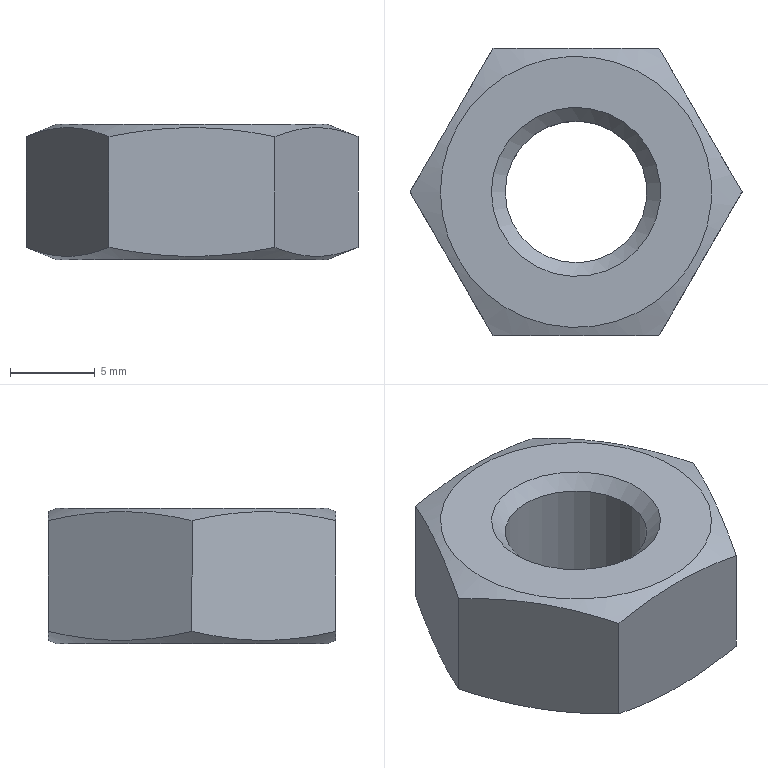Part | STEP file | 1_32 | 1 solid | 13 faces | box 19.63 x 17 x 8 mm | volume 1521 mm3 | plane 8 | cone 4 | cylinder 1 | commonest cylinder face diameters 8.376 x1
STEP:
#1=CARTESIAN_POINT('',(0.,0.,0.));
#2=DIRECTION('',(0.,0.,1.));
#3=DIRECTION('',(1.,0.,0.));
#4=AXIS2_PLACEMENT_3D('',#1,#2,#3);
#5=CARTESIAN_POINT('',(-4.188,0.,0.8119));
#6=VERTEX_POINT('',#5);
#7=CARTESIAN_POINT('',(0.,0.,0.8119));
#8=DIRECTION('',(0.,0.,-1.));
#9=DIRECTION('',(1.,0.,0.));
#10=AXIS2_PLACEMENT_3D('',#7,#8,#9);
#11=CIRCLE('',#10,4.188);
#12=CARTESIAN_POINT('',(0.,0.,0.4059));
#13=DIRECTION('',(0.,0.,-1.));
#14=DIRECTION('',(1.,0.,0.));
#15=AXIS2_PLACEMENT_3D('',#12,#13,#14);
#16=CONICAL_SURFACE('',#15,4.594,0.7854);
#17=CARTESIAN_POINT('',(0.,-0.4059));
#18=DIRECTION('',(1.,0.));
#19=VECTOR('',#18,1.);
#20=LINE('',#17,#19);
#21=(GEOMETRIC_REPRESENTATION_CONTEXT(2)PARAMETRIC_REPRESENTATION_CONTEXT()REPRESENTATION_CONTEXT('',''));
#22=DEFINITIONAL_REPRESENTATION('',(#20),#21);
#23=PCURVE('',#16,#22);
#24=CARTESIAN_POINT('',(0.,0.,4.));
#25=DIRECTION('',(0.,0.,-1.));
#26=DIRECTION('',(1.,0.,0.));
#27=AXIS2_PLACEMENT_3D('',#24,#25,#26);
#28=CYLINDRICAL_SURFACE('',#27,4.188);
#29=CARTESIAN_POINT('',(0.,3.188));
#30=DIRECTION('',(1.,0.));
#31=VECTOR('',#30,1.);
#32=LINE('',#29,#31);
#33=(GEOMETRIC_REPRESENTATION_CONTEXT(2)PARAMETRIC_REPRESENTATION_CONTEXT()REPRESENTATION_CONTEXT('',''));
#34=DEFINITIONAL_REPRESENTATION('',(#32),#33);
#35=PCURVE('',#28,#34);
#36=SURFACE_CURVE('',#11,(#23,#35),.PCURVE_S1.);
#37=EDGE_CURVE('',#6,#6,#36,.T.);
#38=ORIENTED_EDGE('',*,*,#37,.T.);
#39=CARTESIAN_POINT('',(-5.,0.,0.));
#40=VERTEX_POINT('',#39);
#41=CARTESIAN_POINT('',(-4.188,0.,0.8119));
#42=CARTESIAN_POINT('',(-5.,0.,0.));
#43=B_SPLINE_CURVE_WITH_KNOTS('',1,(#41,#42),.UNSPECIFIED.,.F.,.F.,(2,2),(-0.5741,0.5741),.PIECEWISE_BEZIER_KNOTS.);
#44=CARTESIAN_POINT('',(9.425,0.));
#45=DIRECTION('',(0.,1.));
#46=VECTOR('',#45,1.);
#47=LINE('',#44,#46);
#48=(GEOMETRIC_REPRESENTATION_CONTEXT(2)PARAMETRIC_REPRESENTATION_CONTEXT()REPRESENTATION_CONTEXT('',''));
#49=DEFINITIONAL_REPRESENTATION('',(#47),#48);
#50=PCURVE('',#16,#49);
#51=CARTESIAN_POINT('',(3.142,0.));
#52=DIRECTION('',(0.,1.));
#53=VECTOR('',#52,1.);
#54=LINE('',#51,#53);
#55=(GEOMETRIC_REPRESENTATION_CONTEXT(2)PARAMETRIC_REPRESENTATION_CONTEXT()REPRESENTATION_CONTEXT('',''));
#56=DEFINITIONAL_REPRESENTATION('',(#54),#55);
#57=PCURVE('',#16,#56);
#58=SEAM_CURVE('',#43,(#50,#57),.PCURVE_S1.);
#59=EDGE_CURVE('',#6,#40,#58,.T.);
#60=ORIENTED_EDGE('',*,*,#59,.T.);
#61=CARTESIAN_POINT('',(0.,0.,0.));
#62=DIRECTION('',(0.,0.,-1.));
#63=DIRECTION('',(1.,0.,0.));
#64=AXIS2_PLACEMENT_3D('',#61,#62,#63);
#65=CIRCLE('',#64,5.);
#66=CARTESIAN_POINT('',(0.,0.4059));
#67=DIRECTION('',(1.,0.));
#68=VECTOR('',#67,1.);
#69=LINE('',#66,#68);
#70=(GEOMETRIC_REPRESENTATION_CONTEXT(2)PARAMETRIC_REPRESENTATION_CONTEXT()REPRESENTATION_CONTEXT('',''));
#71=DEFINITIONAL_REPRESENTATION('',(#69),#70);
#72=PCURVE('',#16,#71);
#73=CARTESIAN_POINT('',(0.,0.,0.));
#74=DIRECTION('',(0.,0.,1.));
#75=DIRECTION('',(1.,0.,0.));
#76=AXIS2_PLACEMENT_3D('',#73,#74,#75);
#77=PLANE('',#76);
#78=CARTESIAN_POINT('',(5.,0.));
#79=CARTESIAN_POINT('',(5.,-8.66));
#80=CARTESIAN_POINT('',(-2.5,-4.33));
#81=CARTESIAN_POINT('',(-10.,0.));
#82=CARTESIAN_POINT('',(-2.5,4.33));
#83=CARTESIAN_POINT('',(5.,8.66));
#84=CARTESIAN_POINT('',(5.,0.));
#85=(BOUNDED_CURVE()B_SPLINE_CURVE(2,(#78,#79,#80,#81,#82,#83,#84),.UNSPECIFIED.,.T.,.F.)B_SPLINE_CURVE_WITH_KNOTS((1,2,2,2,2,1),(-2.094,0.,2.094,4.189,6.283,8.378),.UNSPECIFIED.)CURVE()GEOMETRIC_REPRESENTATION_ITEM()RATIONAL_B_SPLINE_CURVE((1.,0.5,1.,0.5,1.,0.5,1.))REPRESENTATION_ITEM(''));
#86=(GEOMETRIC_REPRESENTATION_CONTEXT(2)PARAMETRIC_REPRESENTATION_CONTEXT()REPRESENTATION_CONTEXT('',''));
#87=DEFINITIONAL_REPRESENTATION('',(#85),#86);
#88=PCURVE('',#77,#87);
#89=SURFACE_CURVE('',#65,(#72,#88),.PCURVE_S1.);
#90=EDGE_CURVE('',#40,#40,#89,.T.);
#91=ORIENTED_EDGE('',*,*,#90,.F.);
#92=ORIENTED_EDGE('',*,*,#59,.F.);
#93=EDGE_LOOP('',(#38,#60,#91,#92));
#94=FACE_BOUND('',#93,.F.);
#95=ADVANCED_FACE('',(#94),#16,.F.);
#96=CARTESIAN_POINT('',(-8.015,0.,0.));
#97=VERTEX_POINT('',#96);
#98=CARTESIAN_POINT('',(0.,0.,0.));
#99=DIRECTION('',(0.,0.,1.));
#100=DIRECTION('',(1.,0.,0.));
#101=AXIS2_PLACEMENT_3D('',#98,#99,#100);
#102=CIRCLE('',#101,8.015);
#103=CARTESIAN_POINT('',(0.,0.));
#104=DIRECTION('',(1.,0.));
#105=AXIS2_PLACEMENT_2D('',#103,#104);
#106=CIRCLE('',#105,8.015);
#107=(GEOMETRIC_REPRESENTATION_CONTEXT(2)PARAMETRIC_REPRESENTATION_CONTEXT()REPRESENTATION_CONTEXT('',''));
#108=DEFINITIONAL_REPRESENTATION('',(#106),#107);
#109=PCURVE('',#77,#108);
#110=CARTESIAN_POINT('',(0.,0.,0.3636));
#111=DIRECTION('',(0.,0.,1.));
#112=DIRECTION('',(1.,0.,0.));
#113=AXIS2_PLACEMENT_3D('',#110,#111,#112);
#114=CONICAL_SURFACE('',#113,8.915,1.187);
#115=CARTESIAN_POINT('',(0.,-0.3636));
#116=DIRECTION('',(1.,0.));
#117=VECTOR('',#116,1.);
#118=LINE('',#115,#117);
#119=(GEOMETRIC_REPRESENTATION_CONTEXT(2)PARAMETRIC_REPRESENTATION_CONTEXT()REPRESENTATION_CONTEXT('',''));
#120=DEFINITIONAL_REPRESENTATION('',(#118),#119);
#121=PCURVE('',#114,#120);
#122=SURFACE_CURVE('',#102,(#109,#121),.PCURVE_S1.);
#123=EDGE_CURVE('',#97,#97,#122,.T.);
#124=ORIENTED_EDGE('',*,*,#123,.F.);
#125=EDGE_LOOP('',(#124));
#126=FACE_BOUND('',#125,.T.);
#127=ORIENTED_EDGE('',*,*,#90,.F.);
#128=EDGE_LOOP('',(#127));
#129=FACE_BOUND('',#128,.T.);
#130=ADVANCED_FACE('',(#126,#129),#77,.F.);
#131=CARTESIAN_POINT('',(-4.188,0.,7.188));
#132=VERTEX_POINT('',#131);
#133=CARTESIAN_POINT('',(0.,0.,7.188));
#134=DIRECTION('',(0.,0.,1.));
#135=DIRECTION('',(-1.,0.,0.));
#136=AXIS2_PLACEMENT_3D('',#133,#134,#135);
#137=CIRCLE('',#136,4.188);
#138=CARTESIAN_POINT('',(9.425,-3.188));
#139=DIRECTION('',(-1.,0.));
#140=VECTOR('',#139,1.);
#141=LINE('',#138,#140);
#142=(GEOMETRIC_REPRESENTATION_CONTEXT(2)PARAMETRIC_REPRESENTATION_CONTEXT()REPRESENTATION_CONTEXT('',''));
#143=DEFINITIONAL_REPRESENTATION('',(#141),#142);
#144=PCURVE('',#28,#143);
#145=CARTESIAN_POINT('',(0.,0.,7.594));
#146=DIRECTION('',(0.,0.,1.));
#147=DIRECTION('',(-1.,0.,0.));
#148=AXIS2_PLACEMENT_3D('',#145,#146,#147);
#149=CONICAL_SURFACE('',#148,4.594,0.7854);
#150=CARTESIAN_POINT('',(0.,-0.4059));
#151=DIRECTION('',(1.,0.));
#152=VECTOR('',#151,1.);
#153=LINE('',#150,#152);
#154=(GEOMETRIC_REPRESENTATION_CONTEXT(2)PARAMETRIC_REPRESENTATION_CONTEXT()REPRESENTATION_CONTEXT('',''));
#155=DEFINITIONAL_REPRESENTATION('',(#153),#154);
#156=PCURVE('',#149,#155);
#157=SURFACE_CURVE('',#137,(#144,#156),.PCURVE_S1.);
#158=EDGE_CURVE('',#132,#132,#157,.T.);
#159=ORIENTED_EDGE('',*,*,#158,.F.);
#160=CARTESIAN_POINT('',(-4.188,0.,7.188));
#161=CARTESIAN_POINT('',(-4.188,0.,0.8119));
#162=B_SPLINE_CURVE_WITH_KNOTS('',1,(#160,#161),.UNSPECIFIED.,.F.,.F.,(2,2),(-3.188,3.188),.PIECEWISE_BEZIER_KNOTS.);
#163=CARTESIAN_POINT('',(9.425,0.));
#164=DIRECTION('',(0.,1.));
#165=VECTOR('',#164,1.);
#166=LINE('',#163,#165);
#167=(GEOMETRIC_REPRESENTATION_CONTEXT(2)PARAMETRIC_REPRESENTATION_CONTEXT()REPRESENTATION_CONTEXT('',''));
#168=DEFINITIONAL_REPRESENTATION('',(#166),#167);
#169=PCURVE('',#28,#168);
#170=CARTESIAN_POINT('',(3.142,0.));
#171=DIRECTION('',(0.,1.));
#172=VECTOR('',#171,1.);
#173=LINE('',#170,#172);
#174=(GEOMETRIC_REPRESENTATION_CONTEXT(2)PARAMETRIC_REPRESENTATION_CONTEXT()REPRESENTATION_CONTEXT('',''));
#175=DEFINITIONAL_REPRESENTATION('',(#173),#174);
#176=PCURVE('',#28,#175);
#177=SEAM_CURVE('',#162,(#169,#176),.PCURVE_S1.);
#178=EDGE_CURVE('',#132,#6,#177,.T.);
#179=ORIENTED_EDGE('',*,*,#178,.T.);
#180=ORIENTED_EDGE('',*,*,#37,.F.);
#181=ORIENTED_EDGE('',*,*,#178,.F.);
#182=EDGE_LOOP('',(#159,#179,#180,#181));
#183=FACE_BOUND('',#182,.F.);
#184=ADVANCED_FACE('',(#183),#28,.F.);
#185=CARTESIAN_POINT('',(-9.815,0.,0.7273));
#186=VERTEX_POINT('',#185);
#187=CARTESIAN_POINT('',(-4.907,8.5,0.7273));
#188=VERTEX_POINT('',#187);
#189=CARTESIAN_POINT('',(-21.724,-20.628,8.865));
#190=CARTESIAN_POINT('',(-7.361,4.25,-2.264));
#191=CARTESIAN_POINT('',(7.002,29.128,8.865));
#192=(BOUNDED_CURVE()B_SPLINE_CURVE(2,(#189,#190,#191),.UNSPECIFIED.,.F.,.F.)B_SPLINE_CURVE_WITH_KNOTS((3,3),(0.,6.001),.PIECEWISE_BEZIER_KNOTS.)CURVE()GEOMETRIC_REPRESENTATION_ITEM()RATIONAL_B_SPLINE_CURVE((1.,3.524,1.))REPRESENTATION_ITEM(''));
#193=CARTESIAN_POINT('',(9.425,0.3636));
#194=CARTESIAN_POINT('',(9.41,0.329));
#195=CARTESIAN_POINT('',(9.379,0.2637));
#196=CARTESIAN_POINT('',(9.333,0.1773));
#197=CARTESIAN_POINT('',(9.286,0.1018));
#198=CARTESIAN_POINT('',(9.239,0.03643));
#199=CARTESIAN_POINT('',(9.191,-0.01926));
#200=CARTESIAN_POINT('',(9.144,-0.0657));
#201=CARTESIAN_POINT('',(9.095,-0.1032));
#202=CARTESIAN_POINT('',(9.047,-0.1322));
#203=CARTESIAN_POINT('',(8.999,-0.1527));
#204=CARTESIAN_POINT('',(8.95,-0.1649));
#205=CARTESIAN_POINT('',(8.901,-0.169));
#206=CARTESIAN_POINT('',(8.852,-0.1649));
#207=CARTESIAN_POINT('',(8.804,-0.1527));
#208=CARTESIAN_POINT('',(8.755,-0.1322));
#209=CARTESIAN_POINT('',(8.707,-0.1032));
#210=CARTESIAN_POINT('',(8.659,-0.0657));
#211=CARTESIAN_POINT('',(8.611,-0.01926));
#212=CARTESIAN_POINT('',(8.563,0.03643));
#213=CARTESIAN_POINT('',(8.516,0.1018));
#214=CARTESIAN_POINT('',(8.469,0.1773));
#215=CARTESIAN_POINT('',(8.423,0.2637));
#216=CARTESIAN_POINT('',(8.393,0.329));
#217=CARTESIAN_POINT('',(8.378,0.3636));
#218=B_SPLINE_CURVE_WITH_KNOTS('',3,(#193,#194,#195,#196,#197,#198,#199,#200,#201,#202,#203,#204,#205,#206,#207,#208,#209,#210,#211,#212,#213,#214,#215,#216,#217),.UNSPECIFIED.,.F.,.F.,(4,1,1,1,1,1,1,1,1,1,1,1,1,1,1,1,1,1,1,1,1,1,4),(1.924,2.022,2.12,2.218,2.316,2.414,2.511,2.609,2.707,2.805,2.903,3.001,3.098,3.196,3.294,3.392,3.49,3.588,3.686,3.783,3.881,3.979,4.077),.QUASI_UNIFORM_KNOTS.);
#219=(GEOMETRIC_REPRESENTATION_CONTEXT(2)PARAMETRIC_REPRESENTATION_CONTEXT()REPRESENTATION_CONTEXT('',''));
#220=DEFINITIONAL_REPRESENTATION('',(#218),#219);
#221=PCURVE('',#114,#220);
#222=CARTESIAN_POINT('',(-9.815,0.,0.));
#223=DIRECTION('',(-0.866,0.5,0.));
#224=DIRECTION('',(0.,0.,1.));
#225=AXIS2_PLACEMENT_3D('',#222,#223,#224);
#226=PLANE('',#225);
#227=CARTESIAN_POINT('',(8.865,-23.819));
#228=CARTESIAN_POINT('',(-2.264,4.907));
#229=CARTESIAN_POINT('',(8.865,33.634));
#230=(BOUNDED_CURVE()B_SPLINE_CURVE(2,(#227,#228,#229),.UNSPECIFIED.,.F.,.F.)B_SPLINE_CURVE_WITH_KNOTS((3,3),(0.,6.001),.PIECEWISE_BEZIER_KNOTS.)CURVE()GEOMETRIC_REPRESENTATION_ITEM()RATIONAL_B_SPLINE_CURVE((1.,3.524,1.))REPRESENTATION_ITEM(''));
#231=(GEOMETRIC_REPRESENTATION_CONTEXT(2)PARAMETRIC_REPRESENTATION_CONTEXT()REPRESENTATION_CONTEXT('',''));
#232=DEFINITIONAL_REPRESENTATION('',(#230),#231);
#233=PCURVE('',#226,#232);
#234=SURFACE_CURVE('',#192,(#221,#233),.PCURVE_S1.);
#235=EDGE_CURVE('',#186,#188,#234,.T.);
#236=ORIENTED_EDGE('',*,*,#235,.T.);
#237=CARTESIAN_POINT('',(4.907,8.5,0.7273));
#238=VERTEX_POINT('',#237);
#239=CARTESIAN_POINT('',(-28.727,8.5,8.865));
#240=CARTESIAN_POINT('',(0.,8.5,-2.264));
#241=CARTESIAN_POINT('',(28.727,8.5,8.865));
#242=(BOUNDED_CURVE()B_SPLINE_CURVE(2,(#239,#240,#241),.UNSPECIFIED.,.F.,.F.)B_SPLINE_CURVE_WITH_KNOTS((3,3),(0.,6.001),.PIECEWISE_BEZIER_KNOTS.)CURVE()GEOMETRIC_REPRESENTATION_ITEM()RATIONAL_B_SPLINE_CURVE((1.,3.524,1.))REPRESENTATION_ITEM(''));
#243=CARTESIAN_POINT('',(8.378,0.3636));
#244=CARTESIAN_POINT('',(8.362,0.329));
#245=CARTESIAN_POINT('',(8.332,0.2637));
#246=CARTESIAN_POINT('',(8.286,0.1773));
#247=CARTESIAN_POINT('',(8.239,0.1018));
#248=CARTESIAN_POINT('',(8.192,0.03643));
#249=CARTESIAN_POINT('',(8.144,-0.01926));
#250=CARTESIAN_POINT('',(8.096,-0.0657));
#251=CARTESIAN_POINT('',(8.048,-0.1032));
#252=CARTESIAN_POINT('',(8.,-0.1322));
#253=CARTESIAN_POINT('',(7.951,-0.1527));
#254=CARTESIAN_POINT('',(7.903,-0.1649));
#255=CARTESIAN_POINT('',(7.854,-0.169));
#256=CARTESIAN_POINT('',(7.805,-0.1649));
#257=CARTESIAN_POINT('',(7.757,-0.1527));
#258=CARTESIAN_POINT('',(7.708,-0.1322));
#259=CARTESIAN_POINT('',(7.66,-0.1032));
#260=CARTESIAN_POINT('',(7.612,-0.0657));
#261=CARTESIAN_POINT('',(7.564,-0.01926));
#262=CARTESIAN_POINT('',(7.516,0.03643));
#263=CARTESIAN_POINT('',(7.469,0.1018));
#264=CARTESIAN_POINT('',(7.422,0.1773));
#265=CARTESIAN_POINT('',(7.376,0.2637));
#266=CARTESIAN_POINT('',(7.346,0.329));
#267=CARTESIAN_POINT('',(7.33,0.3636));
#268=B_SPLINE_CURVE_WITH_KNOTS('',3,(#243,#244,#245,#246,#247,#248,#249,#250,#251,#252,#253,#254,#255,#256,#257,#258,#259,#260,#261,#262,#263,#264,#265,#266,#267),.UNSPECIFIED.,.F.,.F.,(4,1,1,1,1,1,1,1,1,1,1,1,1,1,1,1,1,1,1,1,1,1,4),(1.924,2.022,2.12,2.218,2.316,2.414,2.511,2.609,2.707,2.805,2.903,3.001,3.098,3.196,3.294,3.392,3.49,3.588,3.686,3.783,3.881,3.979,4.077),.QUASI_UNIFORM_KNOTS.);
#269=(GEOMETRIC_REPRESENTATION_CONTEXT(2)PARAMETRIC_REPRESENTATION_CONTEXT()REPRESENTATION_CONTEXT('',''));
#270=DEFINITIONAL_REPRESENTATION('',(#268),#269);
#271=PCURVE('',#114,#270);
#272=CARTESIAN_POINT('',(-4.907,8.5,0.));
#273=DIRECTION('',(0.,1.,0.));
#274=DIRECTION('',(0.,0.,1.));
#275=AXIS2_PLACEMENT_3D('',#272,#273,#274);
#276=PLANE('',#275);
#277=CARTESIAN_POINT('',(8.865,-23.819));
#278=CARTESIAN_POINT('',(-2.264,4.907));
#279=CARTESIAN_POINT('',(8.865,33.634));
#280=(BOUNDED_CURVE()B_SPLINE_CURVE(2,(#277,#278,#279),.UNSPECIFIED.,.F.,.F.)B_SPLINE_CURVE_WITH_KNOTS((3,3),(0.,6.001),.PIECEWISE_BEZIER_KNOTS.)CURVE()GEOMETRIC_REPRESENTATION_ITEM()RATIONAL_B_SPLINE_CURVE((1.,3.524,1.))REPRESENTATION_ITEM(''));
#281=(GEOMETRIC_REPRESENTATION_CONTEXT(2)PARAMETRIC_REPRESENTATION_CONTEXT()REPRESENTATION_CONTEXT('',''));
#282=DEFINITIONAL_REPRESENTATION('',(#280),#281);
#283=PCURVE('',#276,#282);
#284=SURFACE_CURVE('',#242,(#271,#283),.PCURVE_S1.);
#285=EDGE_CURVE('',#188,#238,#284,.T.);
#286=ORIENTED_EDGE('',*,*,#285,.T.);
#287=CARTESIAN_POINT('',(9.815,0.,0.7273));
#288=VERTEX_POINT('',#287);
#289=CARTESIAN_POINT('',(-7.002,29.128,8.865));
#290=CARTESIAN_POINT('',(7.361,4.25,-2.264));
#291=CARTESIAN_POINT('',(21.724,-20.628,8.865));
#292=(BOUNDED_CURVE()B_SPLINE_CURVE(2,(#289,#290,#291),.UNSPECIFIED.,.F.,.F.)B_SPLINE_CURVE_WITH_KNOTS((3,3),(0.,6.001),.PIECEWISE_BEZIER_KNOTS.)CURVE()GEOMETRIC_REPRESENTATION_ITEM()RATIONAL_B_SPLINE_CURVE((1.,3.524,1.))REPRESENTATION_ITEM(''));
#293=CARTESIAN_POINT('',(7.33,0.3636));
#294=CARTESIAN_POINT('',(7.315,0.329));
#295=CARTESIAN_POINT('',(7.285,0.2637));
#296=CARTESIAN_POINT('',(7.238,0.1773));
#297=CARTESIAN_POINT('',(7.192,0.1018));
#298=CARTESIAN_POINT('',(7.145,0.03643));
#299=CARTESIAN_POINT('',(7.097,-0.01926));
#300=CARTESIAN_POINT('',(7.049,-0.0657));
#301=CARTESIAN_POINT('',(7.001,-0.1032));
#302=CARTESIAN_POINT('',(6.953,-0.1322));
#303=CARTESIAN_POINT('',(6.904,-0.1527));
#304=CARTESIAN_POINT('',(6.856,-0.1649));
#305=CARTESIAN_POINT('',(6.807,-0.169));
#306=CARTESIAN_POINT('',(6.758,-0.1649));
#307=CARTESIAN_POINT('',(6.709,-0.1527));
#308=CARTESIAN_POINT('',(6.661,-0.1322));
#309=CARTESIAN_POINT('',(6.612,-0.1032));
#310=CARTESIAN_POINT('',(6.564,-0.0657));
#311=CARTESIAN_POINT('',(6.516,-0.01926));
#312=CARTESIAN_POINT('',(6.469,0.03643));
#313=CARTESIAN_POINT('',(6.422,0.1018));
#314=CARTESIAN_POINT('',(6.375,0.1773));
#315=CARTESIAN_POINT('',(6.329,0.2637));
#316=CARTESIAN_POINT('',(6.298,0.329));
#317=CARTESIAN_POINT('',(6.283,0.3636));
#318=B_SPLINE_CURVE_WITH_KNOTS('',3,(#293,#294,#295,#296,#297,#298,#299,#300,#301,#302,#303,#304,#305,#306,#307,#308,#309,#310,#311,#312,#313,#314,#315,#316,#317),.UNSPECIFIED.,.F.,.F.,(4,1,1,1,1,1,1,1,1,1,1,1,1,1,1,1,1,1,1,1,1,1,4),(1.924,2.022,2.12,2.218,2.316,2.414,2.511,2.609,2.707,2.805,2.903,3.001,3.098,3.196,3.294,3.392,3.49,3.588,3.686,3.783,3.881,3.979,4.077),.QUASI_UNIFORM_KNOTS.);
#319=(GEOMETRIC_REPRESENTATION_CONTEXT(2)PARAMETRIC_REPRESENTATION_CONTEXT()REPRESENTATION_CONTEXT('',''));
#320=DEFINITIONAL_REPRESENTATION('',(#318),#319);
#321=PCURVE('',#114,#320);
#322=CARTESIAN_POINT('',(4.907,8.5,0.));
#323=DIRECTION('',(0.866,0.5,0.));
#324=DIRECTION('',(0.,0.,-1.));
#325=AXIS2_PLACEMENT_3D('',#322,#323,#324);
#326=PLANE('',#325);
#327=CARTESIAN_POINT('',(-8.865,23.819));
#328=CARTESIAN_POINT('',(2.264,-4.907));
#329=CARTESIAN_POINT('',(-8.865,-33.634));
#330=(BOUNDED_CURVE()B_SPLINE_CURVE(2,(#327,#328,#329),.UNSPECIFIED.,.F.,.F.)B_SPLINE_CURVE_WITH_KNOTS((3,3),(0.,6.001),.PIECEWISE_BEZIER_KNOTS.)CURVE()GEOMETRIC_REPRESENTATION_ITEM()RATIONAL_B_SPLINE_CURVE((1.,3.524,1.))REPRESENTATION_ITEM(''));
#331=(GEOMETRIC_REPRESENTATION_CONTEXT(2)PARAMETRIC_REPRESENTATION_CONTEXT()REPRESENTATION_CONTEXT('',''));
#332=DEFINITIONAL_REPRESENTATION('',(#330),#331);
#333=PCURVE('',#326,#332);
#334=SURFACE_CURVE('',#292,(#321,#333),.PCURVE_S1.);
#335=EDGE_CURVE('',#238,#288,#334,.T.);
#336=ORIENTED_EDGE('',*,*,#335,.T.);
#337=CARTESIAN_POINT('',(4.907,-8.5,0.7273));
#338=VERTEX_POINT('',#337);
#339=CARTESIAN_POINT('',(21.724,20.628,8.865));
#340=CARTESIAN_POINT('',(7.361,-4.25,-2.264));
#341=CARTESIAN_POINT('',(-7.002,-29.128,8.865));
#342=(BOUNDED_CURVE()B_SPLINE_CURVE(2,(#339,#340,#341),.UNSPECIFIED.,.F.,.F.)B_SPLINE_CURVE_WITH_KNOTS((3,3),(0.,6.001),.PIECEWISE_BEZIER_KNOTS.)CURVE()GEOMETRIC_REPRESENTATION_ITEM()RATIONAL_B_SPLINE_CURVE((1.,3.524,1.))REPRESENTATION_ITEM(''));
#343=CARTESIAN_POINT('',(6.283,0.3636));
#344=CARTESIAN_POINT('',(6.268,0.329));
#345=CARTESIAN_POINT('',(6.238,0.2637));
#346=CARTESIAN_POINT('',(6.191,0.1773));
#347=CARTESIAN_POINT('',(6.145,0.1018));
#348=CARTESIAN_POINT('',(6.097,0.03643));
#349=CARTESIAN_POINT('',(6.05,-0.01926));
#350=CARTESIAN_POINT('',(6.002,-0.0657));
#351=CARTESIAN_POINT('',(5.954,-0.1032));
#352=CARTESIAN_POINT('',(5.906,-0.1322));
#353=CARTESIAN_POINT('',(5.857,-0.1527));
#354=CARTESIAN_POINT('',(5.808,-0.1649));
#355=CARTESIAN_POINT('',(5.76,-0.169));
#356=CARTESIAN_POINT('',(5.711,-0.1649));
#357=CARTESIAN_POINT('',(5.662,-0.1527));
#358=CARTESIAN_POINT('',(5.614,-0.1322));
#359=CARTESIAN_POINT('',(5.565,-0.1032));
#360=CARTESIAN_POINT('',(5.517,-0.0657));
#361=CARTESIAN_POINT('',(5.469,-0.01926));
#362=CARTESIAN_POINT('',(5.422,0.03643));
#363=CARTESIAN_POINT('',(5.375,0.1018));
#364=CARTESIAN_POINT('',(5.328,0.1773));
#365=CARTESIAN_POINT('',(5.282,0.2637));
#366=CARTESIAN_POINT('',(5.251,0.329));
#367=CARTESIAN_POINT('',(5.236,0.3636));
#368=B_SPLINE_CURVE_WITH_KNOTS('',3,(#343,#344,#345,#346,#347,#348,#349,#350,#351,#352,#353,#354,#355,#356,#357,#358,#359,#360,#361,#362,#363,#364,#365,#366,#367),.UNSPECIFIED.,.F.,.F.,(4,1,1,1,1,1,1,1,1,1,1,1,1,1,1,1,1,1,1,1,1,1,4),(1.924,2.022,2.12,2.218,2.316,2.414,2.511,2.609,2.707,2.805,2.903,3.001,3.098,3.196,3.294,3.392,3.49,3.588,3.686,3.783,3.881,3.979,4.077),.QUASI_UNIFORM_KNOTS.);
#369=(GEOMETRIC_REPRESENTATION_CONTEXT(2)PARAMETRIC_REPRESENTATION_CONTEXT()REPRESENTATION_CONTEXT('',''));
#370=DEFINITIONAL_REPRESENTATION('',(#368),#369);
#371=PCURVE('',#114,#370);
#372=CARTESIAN_POINT('',(9.815,0.,0.));
#373=DIRECTION('',(0.866,-0.5,0.));
#374=DIRECTION('',(0.,0.,-1.));
#375=AXIS2_PLACEMENT_3D('',#372,#373,#374);
#376=PLANE('',#375);
#377=CARTESIAN_POINT('',(-8.865,23.819));
#378=CARTESIAN_POINT('',(2.264,-4.907));
#379=CARTESIAN_POINT('',(-8.865,-33.634));
#380=(BOUNDED_CURVE()B_SPLINE_CURVE(2,(#377,#378,#379),.UNSPECIFIED.,.F.,.F.)B_SPLINE_CURVE_WITH_KNOTS((3,3),(0.,6.001),.PIECEWISE_BEZIER_KNOTS.)CURVE()GEOMETRIC_REPRESENTATION_ITEM()RATIONAL_B_SPLINE_CURVE((1.,3.524,1.))REPRESENTATION_ITEM(''));
#381=(GEOMETRIC_REPRESENTATION_CONTEXT(2)PARAMETRIC_REPRESENTATION_CONTEXT()REPRESENTATION_CONTEXT('',''));
#382=DEFINITIONAL_REPRESENTATION('',(#380),#381);
#383=PCURVE('',#376,#382);
#384=SURFACE_CURVE('',#342,(#371,#383),.PCURVE_S1.);
#385=EDGE_CURVE('',#288,#338,#384,.T.);
#386=ORIENTED_EDGE('',*,*,#385,.T.);
#387=CARTESIAN_POINT('',(-4.907,-8.5,0.7273));
#388=VERTEX_POINT('',#387);
#389=CARTESIAN_POINT('',(28.727,-8.5,8.865));
#390=CARTESIAN_POINT('',(0.,-8.5,-2.264));
#391=CARTESIAN_POINT('',(-28.727,-8.5,8.865));
#392=(BOUNDED_CURVE()B_SPLINE_CURVE(2,(#389,#390,#391),.UNSPECIFIED.,.F.,.F.)B_SPLINE_CURVE_WITH_KNOTS((3,3),(0.,6.001),.PIECEWISE_BEZIER_KNOTS.)CURVE()GEOMETRIC_REPRESENTATION_ITEM()RATIONAL_B_SPLINE_CURVE((1.,3.524,1.))REPRESENTATION_ITEM(''));
#393=CARTESIAN_POINT('',(5.236,0.3636));
#394=CARTESIAN_POINT('',(5.221,0.329));
#395=CARTESIAN_POINT('',(5.19,0.2637));
#396=CARTESIAN_POINT('',(5.144,0.1773));
#397=CARTESIAN_POINT('',(5.097,0.1018));
#398=CARTESIAN_POINT('',(5.05,0.03643));
#399=CARTESIAN_POINT('',(5.003,-0.01926));
#400=CARTESIAN_POINT('',(4.955,-0.0657));
#401=CARTESIAN_POINT('',(4.907,-0.1032));
#402=CARTESIAN_POINT('',(4.858,-0.1322));
#403=CARTESIAN_POINT('',(4.81,-0.1527));
#404=CARTESIAN_POINT('',(4.761,-0.1649));
#405=CARTESIAN_POINT('',(4.712,-0.169));
#406=CARTESIAN_POINT('',(4.664,-0.1649));
#407=CARTESIAN_POINT('',(4.615,-0.1527));
#408=CARTESIAN_POINT('',(4.566,-0.1322));
#409=CARTESIAN_POINT('',(4.518,-0.1032));
#410=CARTESIAN_POINT('',(4.47,-0.0657));
#411=CARTESIAN_POINT('',(4.422,-0.01926));
#412=CARTESIAN_POINT('',(4.375,0.03643));
#413=CARTESIAN_POINT('',(4.327,0.1018));
#414=CARTESIAN_POINT('',(4.281,0.1773));
#415=CARTESIAN_POINT('',(4.234,0.2637));
#416=CARTESIAN_POINT('',(4.204,0.329));
#417=CARTESIAN_POINT('',(4.189,0.3636));
#418=B_SPLINE_CURVE_WITH_KNOTS('',3,(#393,#394,#395,#396,#397,#398,#399,#400,#401,#402,#403,#404,#405,#406,#407,#408,#409,#410,#411,#412,#413,#414,#415,#416,#417),.UNSPECIFIED.,.F.,.F.,(4,1,1,1,1,1,1,1,1,1,1,1,1,1,1,1,1,1,1,1,1,1,4),(1.924,2.022,2.12,2.218,2.316,2.414,2.511,2.609,2.707,2.805,2.903,3.001,3.098,3.196,3.294,3.392,3.49,3.588,3.686,3.783,3.881,3.979,4.077),.QUASI_UNIFORM_KNOTS.);
#419=(GEOMETRIC_REPRESENTATION_CONTEXT(2)PARAMETRIC_REPRESENTATION_CONTEXT()REPRESENTATION_CONTEXT('',''));
#420=DEFINITIONAL_REPRESENTATION('',(#418),#419);
#421=PCURVE('',#114,#420);
#422=CARTESIAN_POINT('',(4.907,-8.5,0.));
#423=DIRECTION('',(0.,-1.,0.));
#424=DIRECTION('',(0.,0.,-1.));
#425=AXIS2_PLACEMENT_3D('',#422,#423,#424);
#426=PLANE('',#425);
#427=CARTESIAN_POINT('',(-8.865,23.819));
#428=CARTESIAN_POINT('',(2.264,-4.907));
#429=CARTESIAN_POINT('',(-8.865,-33.634));
#430=(BOUNDED_CURVE()B_SPLINE_CURVE(2,(#427,#428,#429),.UNSPECIFIED.,.F.,.F.)B_SPLINE_CURVE_WITH_KNOTS((3,3),(0.,6.001),.PIECEWISE_BEZIER_KNOTS.)CURVE()GEOMETRIC_REPRESENTATION_ITEM()RATIONAL_B_SPLINE_CURVE((1.,3.524,1.))REPRESENTATION_ITEM(''));
#431=(GEOMETRIC_REPRESENTATION_CONTEXT(2)PARAMETRIC_REPRESENTATION_CONTEXT()REPRESENTATION_CONTEXT('',''));
#432=DEFINITIONAL_REPRESENTATION('',(#430),#431);
#433=PCURVE('',#426,#432);
#434=SURFACE_CURVE('',#392,(#421,#433),.PCURVE_S1.);
#435=EDGE_CURVE('',#338,#388,#434,.T.);
#436=ORIENTED_EDGE('',*,*,#435,.T.);
#437=CARTESIAN_POINT('',(7.002,-29.128,8.865));
#438=CARTESIAN_POINT('',(-7.361,-4.25,-2.264));
#439=CARTESIAN_POINT('',(-21.724,20.628,8.865));
#440=(BOUNDED_CURVE()B_SPLINE_CURVE(2,(#437,#438,#439),.UNSPECIFIED.,.F.,.F.)B_SPLINE_CURVE_WITH_KNOTS((3,3),(0.,6.001),.PIECEWISE_BEZIER_KNOTS.)CURVE()GEOMETRIC_REPRESENTATION_ITEM()RATIONAL_B_SPLINE_CURVE((1.,3.524,1.))REPRESENTATION_ITEM(''));
#441=CARTESIAN_POINT('',(4.189,0.3636));
#442=CARTESIAN_POINT('',(4.174,0.329));
#443=CARTESIAN_POINT('',(4.143,0.2637));
#444=CARTESIAN_POINT('',(4.097,0.1773));
#445=CARTESIAN_POINT('',(4.05,0.1018));
#446=CARTESIAN_POINT('',(4.003,0.03643));
#447=CARTESIAN_POINT('',(3.956,-0.01926));
#448=CARTESIAN_POINT('',(3.908,-0.0657));
#449=CARTESIAN_POINT('',(3.859,-0.1032));
#450=CARTESIAN_POINT('',(3.811,-0.1322));
#451=CARTESIAN_POINT('',(3.763,-0.1527));
#452=CARTESIAN_POINT('',(3.714,-0.1649));
#453=CARTESIAN_POINT('',(3.665,-0.169));
#454=CARTESIAN_POINT('',(3.616,-0.1649));
#455=CARTESIAN_POINT('',(3.568,-0.1527));
#456=CARTESIAN_POINT('',(3.519,-0.1322));
#457=CARTESIAN_POINT('',(3.471,-0.1032));
#458=CARTESIAN_POINT('',(3.423,-0.0657));
#459=CARTESIAN_POINT('',(3.375,-0.01926));
#460=CARTESIAN_POINT('',(3.327,0.03643));
#461=CARTESIAN_POINT('',(3.28,0.1018));
#462=CARTESIAN_POINT('',(3.233,0.1773));
#463=CARTESIAN_POINT('',(3.187,0.2637));
#464=CARTESIAN_POINT('',(3.157,0.329));
#465=CARTESIAN_POINT('',(3.142,0.3636));
#466=B_SPLINE_CURVE_WITH_KNOTS('',3,(#441,#442,#443,#444,#445,#446,#447,#448,#449,#450,#451,#452,#453,#454,#455,#456,#457,#458,#459,#460,#461,#462,#463,#464,#465),.UNSPECIFIED.,.F.,.F.,(4,1,1,1,1,1,1,1,1,1,1,1,1,1,1,1,1,1,1,1,1,1,4),(1.924,2.022,2.12,2.218,2.316,2.414,2.511,2.609,2.707,2.805,2.903,3.001,3.098,3.196,3.294,3.392,3.49,3.588,3.686,3.783,3.881,3.979,4.077),.QUASI_UNIFORM_KNOTS.);
#467=(GEOMETRIC_REPRESENTATION_CONTEXT(2)PARAMETRIC_REPRESENTATION_CONTEXT()REPRESENTATION_CONTEXT('',''));
#468=DEFINITIONAL_REPRESENTATION('',(#466),#467);
#469=PCURVE('',#114,#468);
#470=CARTESIAN_POINT('',(-4.907,-8.5,0.));
#471=DIRECTION('',(-0.866,-0.5,0.));
#472=DIRECTION('',(0.,0.,1.));
#473=AXIS2_PLACEMENT_3D('',#470,#471,#472);
#474=PLANE('',#473);
#475=CARTESIAN_POINT('',(8.865,-23.819));
#476=CARTESIAN_POINT('',(-2.264,4.907));
#477=CARTESIAN_POINT('',(8.865,33.634));
#478=(BOUNDED_CURVE()B_SPLINE_CURVE(2,(#475,#476,#477),.UNSPECIFIED.,.F.,.F.)B_SPLINE_CURVE_WITH_KNOTS((3,3),(0.,6.001),.PIECEWISE_BEZIER_KNOTS.)CURVE()GEOMETRIC_REPRESENTATION_ITEM()RATIONAL_B_SPLINE_CURVE((1.,3.524,1.))REPRESENTATION_ITEM(''));
#479=(GEOMETRIC_REPRESENTATION_CONTEXT(2)PARAMETRIC_REPRESENTATION_CONTEXT()REPRESENTATION_CONTEXT('',''));
#480=DEFINITIONAL_REPRESENTATION('',(#478),#479);
#481=PCURVE('',#474,#480);
#482=SURFACE_CURVE('',#440,(#469,#481),.PCURVE_S1.);
#483=EDGE_CURVE('',#388,#186,#482,.T.);
#484=ORIENTED_EDGE('',*,*,#483,.T.);
#485=CARTESIAN_POINT('',(-8.015,0.,-0.000000001));
#486=CARTESIAN_POINT('',(-9.815,0.,0.7273));
#487=B_SPLINE_CURVE_WITH_KNOTS('',1,(#485,#486),.UNSPECIFIED.,.F.,.F.,(2,2),(-0.9707,0.9707),.PIECEWISE_BEZIER_KNOTS.);
#488=CARTESIAN_POINT('',(3.142,0.));
#489=DIRECTION('',(0.,1.));
#490=VECTOR('',#489,1.);
#491=LINE('',#488,#490);
#492=(GEOMETRIC_REPRESENTATION_CONTEXT(2)PARAMETRIC_REPRESENTATION_CONTEXT()REPRESENTATION_CONTEXT('',''));
#493=DEFINITIONAL_REPRESENTATION('',(#491),#492);
#494=PCURVE('',#114,#493);
#495=CARTESIAN_POINT('',(9.425,0.));
#496=DIRECTION('',(0.,1.));
#497=VECTOR('',#496,1.);
#498=LINE('',#495,#497);
#499=(GEOMETRIC_REPRESENTATION_CONTEXT(2)PARAMETRIC_REPRESENTATION_CONTEXT()REPRESENTATION_CONTEXT('',''));
#500=DEFINITIONAL_REPRESENTATION('',(#498),#499);
#501=PCURVE('',#114,#500);
#502=SEAM_CURVE('',#487,(#494,#501),.PCURVE_S1.);
#503=EDGE_CURVE('',#97,#186,#502,.T.);
#504=ORIENTED_EDGE('',*,*,#503,.F.);
#505=ORIENTED_EDGE('',*,*,#123,.T.);
#506=ORIENTED_EDGE('',*,*,#503,.T.);
#507=EDGE_LOOP('',(#236,#286,#336,#386,#436,#484,#504,#505,#506));
#508=FACE_BOUND('',#507,.T.);
#509=ADVANCED_FACE('',(#508),#114,.T.);
#510=CARTESIAN_POINT('',(-5.,0.,8.));
#511=VERTEX_POINT('',#510);
#512=CARTESIAN_POINT('',(0.,0.,8.));
#513=DIRECTION('',(0.,0.,1.));
#514=DIRECTION('',(1.,0.,0.));
#515=AXIS2_PLACEMENT_3D('',#512,#513,#514);
#516=CIRCLE('',#515,5.);
#517=CARTESIAN_POINT('',(-3.142,0.4059));
#518=DIRECTION('',(1.,0.));
#519=VECTOR('',#518,1.);
#520=LINE('',#517,#519);
#521=(GEOMETRIC_REPRESENTATION_CONTEXT(2)PARAMETRIC_REPRESENTATION_CONTEXT()REPRESENTATION_CONTEXT('',''));
#522=DEFINITIONAL_REPRESENTATION('',(#520),#521);
#523=PCURVE('',#149,#522);
#524=CARTESIAN_POINT('',(0.,0.,8.));
#525=DIRECTION('',(0.,0.,1.));
#526=DIRECTION('',(1.,0.,0.));
#527=AXIS2_PLACEMENT_3D('',#524,#525,#526);
#528=PLANE('',#527);
#529=CARTESIAN_POINT('',(0.,0.));
#530=DIRECTION('',(1.,0.));
#531=AXIS2_PLACEMENT_2D('',#529,#530);
#532=CIRCLE('',#531,5.);
#533=(GEOMETRIC_REPRESENTATION_CONTEXT(2)PARAMETRIC_REPRESENTATION_CONTEXT()REPRESENTATION_CONTEXT('',''));
#534=DEFINITIONAL_REPRESENTATION('',(#532),#533);
#535=PCURVE('',#528,#534);
#536=SURFACE_CURVE('',#516,(#523,#535),.PCURVE_S1.);
#537=EDGE_CURVE('',#511,#511,#536,.T.);
#538=ORIENTED_EDGE('',*,*,#537,.F.);
#539=CARTESIAN_POINT('',(-4.188,0.,7.188));
#540=CARTESIAN_POINT('',(-5.,0.,8.));
#541=B_SPLINE_CURVE_WITH_KNOTS('',1,(#539,#540),.UNSPECIFIED.,.F.,.F.,(2,2),(-0.5741,0.5741),.PIECEWISE_BEZIER_KNOTS.);
#542=CARTESIAN_POINT('',(0.,0.));
#543=DIRECTION('',(0.,1.));
#544=VECTOR('',#543,1.);
#545=LINE('',#542,#544);
#546=(GEOMETRIC_REPRESENTATION_CONTEXT(2)PARAMETRIC_REPRESENTATION_CONTEXT()REPRESENTATION_CONTEXT('',''));
#547=DEFINITIONAL_REPRESENTATION('',(#545),#546);
#548=PCURVE('',#149,#547);
#549=CARTESIAN_POINT('',(6.283,0.));
#550=DIRECTION('',(0.,1.));
#551=VECTOR('',#550,1.);
#552=LINE('',#549,#551);
#553=(GEOMETRIC_REPRESENTATION_CONTEXT(2)PARAMETRIC_REPRESENTATION_CONTEXT()REPRESENTATION_CONTEXT('',''));
#554=DEFINITIONAL_REPRESENTATION('',(#552),#553);
#555=PCURVE('',#149,#554);
#556=SEAM_CURVE('',#541,(#548,#555),.PCURVE_S1.);
#557=EDGE_CURVE('',#132,#511,#556,.T.);
#558=ORIENTED_EDGE('',*,*,#557,.F.);
#559=ORIENTED_EDGE('',*,*,#158,.T.);
#560=ORIENTED_EDGE('',*,*,#557,.T.);
#561=EDGE_LOOP('',(#538,#558,#559,#560));
#562=FACE_BOUND('',#561,.F.);
#563=ADVANCED_FACE('',(#562),#149,.F.);
#564=CARTESIAN_POINT('',(-4.907,8.5,7.273));
#565=VERTEX_POINT('',#564);
#566=CARTESIAN_POINT('',(-9.815,0.,7.273));
#567=VERTEX_POINT('',#566);
#568=CARTESIAN_POINT('',(7.516,30.018,-1.264));
#569=CARTESIAN_POINT('',(-7.361,4.25,10.295));
#570=CARTESIAN_POINT('',(-22.238,-21.518,-1.264));
#571=(BOUNDED_CURVE()B_SPLINE_CURVE(2,(#568,#569,#570),.UNSPECIFIED.,.F.,.F.)B_SPLINE_CURVE_WITH_KNOTS((3,3),(0.,6.221),.PIECEWISE_BEZIER_KNOTS.)CURVE()GEOMETRIC_REPRESENTATION_ITEM()RATIONAL_B_SPLINE_CURVE((1.,3.641,1.))REPRESENTATION_ITEM(''));
#572=CARTESIAN_POINT('',(-1.264,34.662));
#573=CARTESIAN_POINT('',(10.295,4.907));
#574=CARTESIAN_POINT('',(-1.264,-24.847));
#575=(BOUNDED_CURVE()B_SPLINE_CURVE(2,(#572,#573,#574),.UNSPECIFIED.,.F.,.F.)B_SPLINE_CURVE_WITH_KNOTS((3,3),(0.,6.221),.PIECEWISE_BEZIER_KNOTS.)CURVE()GEOMETRIC_REPRESENTATION_ITEM()RATIONAL_B_SPLINE_CURVE((1.,3.641,1.))REPRESENTATION_ITEM(''));
#576=(GEOMETRIC_REPRESENTATION_CONTEXT(2)PARAMETRIC_REPRESENTATION_CONTEXT()REPRESENTATION_CONTEXT('',''));
#577=DEFINITIONAL_REPRESENTATION('',(#575),#576);
#578=PCURVE('',#226,#577);
#579=CARTESIAN_POINT('',(0.,0.,7.636));
#580=DIRECTION('',(0.,0.,-1.));
#581=DIRECTION('',(-1.,0.,0.));
#582=AXIS2_PLACEMENT_3D('',#579,#580,#581);
#583=CONICAL_SURFACE('',#582,8.915,1.187);
#584=CARTESIAN_POINT('',(1.047,0.3636));
#585=CARTESIAN_POINT('',(1.032,0.329));
#586=CARTESIAN_POINT('',(1.002,0.2637));
#587=CARTESIAN_POINT('',(0.9553,0.1773));
#588=CARTESIAN_POINT('',(0.9086,0.1018));
#589=CARTESIAN_POINT('',(0.8614,0.03643));
#590=CARTESIAN_POINT('',(0.8139,-0.01926));
#591=CARTESIAN_POINT('',(0.766,-0.0657));
#592=CARTESIAN_POINT('',(0.7179,-0.1032));
#593=CARTESIAN_POINT('',(0.6695,-0.1322));
#594=CARTESIAN_POINT('',(0.621,-0.1527));
#595=CARTESIAN_POINT('',(0.5723,-0.1649));
#596=CARTESIAN_POINT('',(0.5236,-0.169));
#597=CARTESIAN_POINT('',(0.4749,-0.1649));
#598=CARTESIAN_POINT('',(0.4262,-0.1527));
#599=CARTESIAN_POINT('',(0.3777,-0.1322));
#600=CARTESIAN_POINT('',(0.3293,-0.1032));
#601=CARTESIAN_POINT('',(0.2812,-0.0657));
#602=CARTESIAN_POINT('',(0.2333,-0.01926));
#603=CARTESIAN_POINT('',(0.1858,0.03643));
#604=CARTESIAN_POINT('',(0.1386,0.1018));
#605=CARTESIAN_POINT('',(0.09189,0.1773));
#606=CARTESIAN_POINT('',(0.04564,0.2637));
#607=CARTESIAN_POINT('',(0.01515,0.329));
#608=CARTESIAN_POINT('',(0.,0.3636));
#609=B_SPLINE_CURVE_WITH_KNOTS('',3,(#584,#585,#586,#587,#588,#589,#590,#591,#592,#593,#594,#595,#596,#597,#598,#599,#600,#601,#602,#603,#604,#605,#606,#607,#608),.UNSPECIFIED.,.F.,.F.,(4,1,1,1,1,1,1,1,1,1,1,1,1,1,1,1,1,1,1,1,1,1,4),(2.006,2.106,2.207,2.307,2.407,2.508,2.608,2.709,2.809,2.91,3.01,3.111,3.211,3.311,3.412,3.512,3.613,3.713,3.814,3.914,4.015,4.115,4.215),.QUASI_UNIFORM_KNOTS.);
#610=(GEOMETRIC_REPRESENTATION_CONTEXT(2)PARAMETRIC_REPRESENTATION_CONTEXT()REPRESENTATION_CONTEXT('',''));
#611=DEFINITIONAL_REPRESENTATION('',(#609),#610);
#612=PCURVE('',#583,#611);
#613=SURFACE_CURVE('',#571,(#578,#612),.PCURVE_S1.);
#614=EDGE_CURVE('',#565,#567,#613,.T.);
#615=ORIENTED_EDGE('',*,*,#614,.F.);
#616=CARTESIAN_POINT('',(-4.907,8.5,0.7273));
#617=DIRECTION('',(0.,0.,1.));
#618=VECTOR('',#617,1.);
#619=LINE('',#616,#618);
#620=CARTESIAN_POINT('',(0.7273,9.815));
#621=DIRECTION('',(1.,0.));
#622=VECTOR('',#621,1.);
#623=LINE('',#620,#622);
#624=(GEOMETRIC_REPRESENTATION_CONTEXT(2)PARAMETRIC_REPRESENTATION_CONTEXT()REPRESENTATION_CONTEXT('',''));
#625=DEFINITIONAL_REPRESENTATION('',(#623),#624);
#626=PCURVE('',#226,#625);
#627=CARTESIAN_POINT('',(0.7273,0.));
#628=DIRECTION('',(1.,0.));
#629=VECTOR('',#628,1.);
#630=LINE('',#627,#629);
#631=(GEOMETRIC_REPRESENTATION_CONTEXT(2)PARAMETRIC_REPRESENTATION_CONTEXT()REPRESENTATION_CONTEXT('',''));
#632=DEFINITIONAL_REPRESENTATION('',(#630),#631);
#633=PCURVE('',#276,#632);
#634=SURFACE_CURVE('',#619,(#626,#633),.PCURVE_S1.);
#635=EDGE_CURVE('',#188,#565,#634,.T.);
#636=ORIENTED_EDGE('',*,*,#635,.F.);
#637=ORIENTED_EDGE('',*,*,#235,.F.);
#638=CARTESIAN_POINT('',(-9.815,0.,0.7273));
#639=DIRECTION('',(0.,0.,1.));
#640=VECTOR('',#639,1.);
#641=LINE('',#638,#640);
#642=CARTESIAN_POINT('',(0.7273,0.));
#643=DIRECTION('',(1.,0.));
#644=VECTOR('',#643,1.);
#645=LINE('',#642,#644);
#646=(GEOMETRIC_REPRESENTATION_CONTEXT(2)PARAMETRIC_REPRESENTATION_CONTEXT()REPRESENTATION_CONTEXT('',''));
#647=DEFINITIONAL_REPRESENTATION('',(#645),#646);
#648=PCURVE('',#226,#647);
#649=CARTESIAN_POINT('',(0.7273,9.815));
#650=DIRECTION('',(1.,0.));
#651=VECTOR('',#650,1.);
#652=LINE('',#649,#651);
#653=(GEOMETRIC_REPRESENTATION_CONTEXT(2)PARAMETRIC_REPRESENTATION_CONTEXT()REPRESENTATION_CONTEXT('',''));
#654=DEFINITIONAL_REPRESENTATION('',(#652),#653);
#655=PCURVE('',#474,#654);
#656=SURFACE_CURVE('',#641,(#648,#655),.PCURVE_S1.);
#657=EDGE_CURVE('',#186,#567,#656,.T.);
#658=ORIENTED_EDGE('',*,*,#657,.T.);
#659=EDGE_LOOP('',(#615,#636,#637,#658));
#660=FACE_BOUND('',#659,.T.);
#661=ADVANCED_FACE('',(#660),#226,.T.);
#662=CARTESIAN_POINT('',(4.907,8.5,7.273));
#663=VERTEX_POINT('',#662);
#664=CARTESIAN_POINT('',(29.754,8.5,-1.264));
#665=CARTESIAN_POINT('',(0.,8.5,10.295));
#666=CARTESIAN_POINT('',(-29.754,8.5,-1.264));
#667=(BOUNDED_CURVE()B_SPLINE_CURVE(2,(#664,#665,#666),.UNSPECIFIED.,.F.,.F.)B_SPLINE_CURVE_WITH_KNOTS((3,3),(0.,6.221),.PIECEWISE_BEZIER_KNOTS.)CURVE()GEOMETRIC_REPRESENTATION_ITEM()RATIONAL_B_SPLINE_CURVE((1.,3.641,1.))REPRESENTATION_ITEM(''));
#668=CARTESIAN_POINT('',(-1.264,34.662));
#669=CARTESIAN_POINT('',(10.295,4.907));
#670=CARTESIAN_POINT('',(-1.264,-24.847));
#671=(BOUNDED_CURVE()B_SPLINE_CURVE(2,(#668,#669,#670),.UNSPECIFIED.,.F.,.F.)B_SPLINE_CURVE_WITH_KNOTS((3,3),(0.,6.221),.PIECEWISE_BEZIER_KNOTS.)CURVE()GEOMETRIC_REPRESENTATION_ITEM()RATIONAL_B_SPLINE_CURVE((1.,3.641,1.))REPRESENTATION_ITEM(''));
#672=(GEOMETRIC_REPRESENTATION_CONTEXT(2)PARAMETRIC_REPRESENTATION_CONTEXT()REPRESENTATION_CONTEXT('',''));
#673=DEFINITIONAL_REPRESENTATION('',(#671),#672);
#674=PCURVE('',#276,#673);
#675=CARTESIAN_POINT('',(2.094,0.3636));
#676=CARTESIAN_POINT('',(2.079,0.329));
#677=CARTESIAN_POINT('',(2.049,0.2637));
#678=CARTESIAN_POINT('',(2.003,0.1773));
#679=CARTESIAN_POINT('',(1.956,0.1018));
#680=CARTESIAN_POINT('',(1.909,0.03643));
#681=CARTESIAN_POINT('',(1.861,-0.01926));
#682=CARTESIAN_POINT('',(1.813,-0.0657));
#683=CARTESIAN_POINT('',(1.765,-0.1032));
#684=CARTESIAN_POINT('',(1.717,-0.1322));
#685=CARTESIAN_POINT('',(1.668,-0.1527));
#686=CARTESIAN_POINT('',(1.62,-0.1649));
#687=CARTESIAN_POINT('',(1.571,-0.169));
#688=CARTESIAN_POINT('',(1.522,-0.1649));
#689=CARTESIAN_POINT('',(1.473,-0.1527));
#690=CARTESIAN_POINT('',(1.425,-0.1322));
#691=CARTESIAN_POINT('',(1.376,-0.1032));
#692=CARTESIAN_POINT('',(1.328,-0.0657));
#693=CARTESIAN_POINT('',(1.28,-0.01926));
#694=CARTESIAN_POINT('',(1.233,0.03643));
#695=CARTESIAN_POINT('',(1.186,0.1018));
#696=CARTESIAN_POINT('',(1.139,0.1773));
#697=CARTESIAN_POINT('',(1.093,0.2637));
#698=CARTESIAN_POINT('',(1.062,0.329));
#699=CARTESIAN_POINT('',(1.047,0.3636));
#700=B_SPLINE_CURVE_WITH_KNOTS('',3,(#675,#676,#677,#678,#679,#680,#681,#682,#683,#684,#685,#686,#687,#688,#689,#690,#691,#692,#693,#694,#695,#696,#697,#698,#699),.UNSPECIFIED.,.F.,.F.,(4,1,1,1,1,1,1,1,1,1,1,1,1,1,1,1,1,1,1,1,1,1,4),(2.006,2.106,2.207,2.307,2.407,2.508,2.608,2.709,2.809,2.91,3.01,3.111,3.211,3.311,3.412,3.512,3.613,3.713,3.814,3.914,4.015,4.115,4.215),.QUASI_UNIFORM_KNOTS.);
#701=(GEOMETRIC_REPRESENTATION_CONTEXT(2)PARAMETRIC_REPRESENTATION_CONTEXT()REPRESENTATION_CONTEXT('',''));
#702=DEFINITIONAL_REPRESENTATION('',(#700),#701);
#703=PCURVE('',#583,#702);
#704=SURFACE_CURVE('',#667,(#674,#703),.PCURVE_S1.);
#705=EDGE_CURVE('',#663,#565,#704,.T.);
#706=ORIENTED_EDGE('',*,*,#705,.F.);
#707=CARTESIAN_POINT('',(4.907,8.5,0.7273));
#708=DIRECTION('',(0.,0.,1.));
#709=VECTOR('',#708,1.);
#710=LINE('',#707,#709);
#711=CARTESIAN_POINT('',(0.7273,9.815));
#712=DIRECTION('',(1.,0.));
#713=VECTOR('',#712,1.);
#714=LINE('',#711,#713);
#715=(GEOMETRIC_REPRESENTATION_CONTEXT(2)PARAMETRIC_REPRESENTATION_CONTEXT()REPRESENTATION_CONTEXT('',''));
#716=DEFINITIONAL_REPRESENTATION('',(#714),#715);
#717=PCURVE('',#276,#716);
#718=CARTESIAN_POINT('',(-0.7273,0.));
#719=DIRECTION('',(-1.,0.));
#720=VECTOR('',#719,1.);
#721=LINE('',#718,#720);
#722=(GEOMETRIC_REPRESENTATION_CONTEXT(2)PARAMETRIC_REPRESENTATION_CONTEXT()REPRESENTATION_CONTEXT('',''));
#723=DEFINITIONAL_REPRESENTATION('',(#721),#722);
#724=PCURVE('',#326,#723);
#725=SURFACE_CURVE('',#710,(#717,#724),.PCURVE_S1.);
#726=EDGE_CURVE('',#238,#663,#725,.T.);
#727=ORIENTED_EDGE('',*,*,#726,.F.);
#728=ORIENTED_EDGE('',*,*,#285,.F.);
#729=ORIENTED_EDGE('',*,*,#635,.T.);
#730=EDGE_LOOP('',(#706,#727,#728,#729));
#731=FACE_BOUND('',#730,.T.);
#732=ADVANCED_FACE('',(#731),#276,.T.);
#733=CARTESIAN_POINT('',(9.815,0.,7.273));
#734=VERTEX_POINT('',#733);
#735=CARTESIAN_POINT('',(22.238,-21.518,-1.264));
#736=CARTESIAN_POINT('',(7.361,4.25,10.295));
#737=CARTESIAN_POINT('',(-7.516,30.018,-1.264));
#738=(BOUNDED_CURVE()B_SPLINE_CURVE(2,(#735,#736,#737),.UNSPECIFIED.,.F.,.F.)B_SPLINE_CURVE_WITH_KNOTS((3,3),(0.,6.221),.PIECEWISE_BEZIER_KNOTS.)CURVE()GEOMETRIC_REPRESENTATION_ITEM()RATIONAL_B_SPLINE_CURVE((1.,3.641,1.))REPRESENTATION_ITEM(''));
#739=CARTESIAN_POINT('',(1.264,-34.662));
#740=CARTESIAN_POINT('',(-10.295,-4.907));
#741=CARTESIAN_POINT('',(1.264,24.847));
#742=(BOUNDED_CURVE()B_SPLINE_CURVE(2,(#739,#740,#741),.UNSPECIFIED.,.F.,.F.)B_SPLINE_CURVE_WITH_KNOTS((3,3),(0.,6.221),.PIECEWISE_BEZIER_KNOTS.)CURVE()GEOMETRIC_REPRESENTATION_ITEM()RATIONAL_B_SPLINE_CURVE((1.,3.641,1.))REPRESENTATION_ITEM(''));
#743=(GEOMETRIC_REPRESENTATION_CONTEXT(2)PARAMETRIC_REPRESENTATION_CONTEXT()REPRESENTATION_CONTEXT('',''));
#744=DEFINITIONAL_REPRESENTATION('',(#742),#743);
#745=PCURVE('',#326,#744);
#746=CARTESIAN_POINT('',(3.142,0.3636));
#747=CARTESIAN_POINT('',(3.126,0.329));
#748=CARTESIAN_POINT('',(3.096,0.2637));
#749=CARTESIAN_POINT('',(3.05,0.1773));
#750=CARTESIAN_POINT('',(3.003,0.1018));
#751=CARTESIAN_POINT('',(2.956,0.03643));
#752=CARTESIAN_POINT('',(2.908,-0.01926));
#753=CARTESIAN_POINT('',(2.86,-0.0657));
#754=CARTESIAN_POINT('',(2.812,-0.1032));
#755=CARTESIAN_POINT('',(2.764,-0.1322));
#756=CARTESIAN_POINT('',(2.715,-0.1527));
#757=CARTESIAN_POINT('',(2.667,-0.1649));
#758=CARTESIAN_POINT('',(2.618,-0.169));
#759=CARTESIAN_POINT('',(2.569,-0.1649));
#760=CARTESIAN_POINT('',(2.521,-0.1527));
#761=CARTESIAN_POINT('',(2.472,-0.1322));
#762=CARTESIAN_POINT('',(2.424,-0.1032));
#763=CARTESIAN_POINT('',(2.376,-0.0657));
#764=CARTESIAN_POINT('',(2.328,-0.01926));
#765=CARTESIAN_POINT('',(2.28,0.03643));
#766=CARTESIAN_POINT('',(2.233,0.1018));
#767=CARTESIAN_POINT('',(2.186,0.1773));
#768=CARTESIAN_POINT('',(2.14,0.2637));
#769=CARTESIAN_POINT('',(2.11,0.329));
#770=CARTESIAN_POINT('',(2.094,0.3636));
#771=B_SPLINE_CURVE_WITH_KNOTS('',3,(#746,#747,#748,#749,#750,#751,#752,#753,#754,#755,#756,#757,#758,#759,#760,#761,#762,#763,#764,#765,#766,#767,#768,#769,#770),.UNSPECIFIED.,.F.,.F.,(4,1,1,1,1,1,1,1,1,1,1,1,1,1,1,1,1,1,1,1,1,1,4),(2.006,2.106,2.207,2.307,2.407,2.508,2.608,2.709,2.809,2.91,3.01,3.111,3.211,3.311,3.412,3.512,3.613,3.713,3.814,3.914,4.015,4.115,4.215),.QUASI_UNIFORM_KNOTS.);
#772=(GEOMETRIC_REPRESENTATION_CONTEXT(2)PARAMETRIC_REPRESENTATION_CONTEXT()REPRESENTATION_CONTEXT('',''));
#773=DEFINITIONAL_REPRESENTATION('',(#771),#772);
#774=PCURVE('',#583,#773);
#775=SURFACE_CURVE('',#738,(#745,#774),.PCURVE_S1.);
#776=EDGE_CURVE('',#734,#663,#775,.T.);
#777=ORIENTED_EDGE('',*,*,#776,.F.);
#778=CARTESIAN_POINT('',(9.815,0.,0.7273));
#779=DIRECTION('',(0.,0.,1.));
#780=VECTOR('',#779,1.);
#781=LINE('',#778,#780);
#782=CARTESIAN_POINT('',(-0.7273,-9.815));
#783=DIRECTION('',(-1.,0.));
#784=VECTOR('',#783,1.);
#785=LINE('',#782,#784);
#786=(GEOMETRIC_REPRESENTATION_CONTEXT(2)PARAMETRIC_REPRESENTATION_CONTEXT()REPRESENTATION_CONTEXT('',''));
#787=DEFINITIONAL_REPRESENTATION('',(#785),#786);
#788=PCURVE('',#326,#787);
#789=CARTESIAN_POINT('',(-0.7273,0.));
#790=DIRECTION('',(-1.,0.));
#791=VECTOR('',#790,1.);
#792=LINE('',#789,#791);
#793=(GEOMETRIC_REPRESENTATION_CONTEXT(2)PARAMETRIC_REPRESENTATION_CONTEXT()REPRESENTATION_CONTEXT('',''));
#794=DEFINITIONAL_REPRESENTATION('',(#792),#793);
#795=PCURVE('',#376,#794);
#796=SURFACE_CURVE('',#781,(#788,#795),.PCURVE_S1.);
#797=EDGE_CURVE('',#288,#734,#796,.T.);
#798=ORIENTED_EDGE('',*,*,#797,.F.);
#799=ORIENTED_EDGE('',*,*,#335,.F.);
#800=ORIENTED_EDGE('',*,*,#726,.T.);
#801=EDGE_LOOP('',(#777,#798,#799,#800));
#802=FACE_BOUND('',#801,.T.);
#803=ADVANCED_FACE('',(#802),#326,.T.);
#804=CARTESIAN_POINT('',(4.907,-8.5,7.273));
#805=VERTEX_POINT('',#804);
#806=CARTESIAN_POINT('',(-7.516,-30.018,-1.264));
#807=CARTESIAN_POINT('',(7.361,-4.25,10.295));
#808=CARTESIAN_POINT('',(22.238,21.518,-1.264));
#809=(BOUNDED_CURVE()B_SPLINE_CURVE(2,(#806,#807,#808),.UNSPECIFIED.,.F.,.F.)B_SPLINE_CURVE_WITH_KNOTS((3,3),(0.,6.221),.PIECEWISE_BEZIER_KNOTS.)CURVE()GEOMETRIC_REPRESENTATION_ITEM()RATIONAL_B_SPLINE_CURVE((1.,3.641,1.))REPRESENTATION_ITEM(''));
#810=CARTESIAN_POINT('',(1.264,-34.662));
#811=CARTESIAN_POINT('',(-10.295,-4.907));
#812=CARTESIAN_POINT('',(1.264,24.847));
#813=(BOUNDED_CURVE()B_SPLINE_CURVE(2,(#810,#811,#812),.UNSPECIFIED.,.F.,.F.)B_SPLINE_CURVE_WITH_KNOTS((3,3),(0.,6.221),.PIECEWISE_BEZIER_KNOTS.)CURVE()GEOMETRIC_REPRESENTATION_ITEM()RATIONAL_B_SPLINE_CURVE((1.,3.641,1.))REPRESENTATION_ITEM(''));
#814=(GEOMETRIC_REPRESENTATION_CONTEXT(2)PARAMETRIC_REPRESENTATION_CONTEXT()REPRESENTATION_CONTEXT('',''));
#815=DEFINITIONAL_REPRESENTATION('',(#813),#814);
#816=PCURVE('',#376,#815);
#817=CARTESIAN_POINT('',(4.189,0.3636));
#818=CARTESIAN_POINT('',(4.174,0.329));
#819=CARTESIAN_POINT('',(4.143,0.2637));
#820=CARTESIAN_POINT('',(4.097,0.1773));
#821=CARTESIAN_POINT('',(4.05,0.1018));
#822=CARTESIAN_POINT('',(4.003,0.03643));
#823=CARTESIAN_POINT('',(3.956,-0.01926));
#824=CARTESIAN_POINT('',(3.908,-0.0657));
#825=CARTESIAN_POINT('',(3.859,-0.1032));
#826=CARTESIAN_POINT('',(3.811,-0.1322));
#827=CARTESIAN_POINT('',(3.763,-0.1527));
#828=CARTESIAN_POINT('',(3.714,-0.1649));
#829=CARTESIAN_POINT('',(3.665,-0.169));
#830=CARTESIAN_POINT('',(3.616,-0.1649));
#831=CARTESIAN_POINT('',(3.568,-0.1527));
#832=CARTESIAN_POINT('',(3.519,-0.1322));
#833=CARTESIAN_POINT('',(3.471,-0.1032));
#834=CARTESIAN_POINT('',(3.423,-0.0657));
#835=CARTESIAN_POINT('',(3.375,-0.01926));
#836=CARTESIAN_POINT('',(3.327,0.03643));
#837=CARTESIAN_POINT('',(3.28,0.1018));
#838=CARTESIAN_POINT('',(3.233,0.1773));
#839=CARTESIAN_POINT('',(3.187,0.2637));
#840=CARTESIAN_POINT('',(3.157,0.329));
#841=CARTESIAN_POINT('',(3.142,0.3636));
#842=B_SPLINE_CURVE_WITH_KNOTS('',3,(#817,#818,#819,#820,#821,#822,#823,#824,#825,#826,#827,#828,#829,#830,#831,#832,#833,#834,#835,#836,#837,#838,#839,#840,#841),.UNSPECIFIED.,.F.,.F.,(4,1,1,1,1,1,1,1,1,1,1,1,1,1,1,1,1,1,1,1,1,1,4),(2.006,2.106,2.207,2.307,2.407,2.508,2.608,2.709,2.809,2.91,3.01,3.111,3.211,3.311,3.412,3.512,3.613,3.713,3.814,3.914,4.015,4.115,4.215),.QUASI_UNIFORM_KNOTS.);
#843=(GEOMETRIC_REPRESENTATION_CONTEXT(2)PARAMETRIC_REPRESENTATION_CONTEXT()REPRESENTATION_CONTEXT('',''));
#844=DEFINITIONAL_REPRESENTATION('',(#842),#843);
#845=PCURVE('',#583,#844);
#846=SURFACE_CURVE('',#809,(#816,#845),.PCURVE_S1.);
#847=EDGE_CURVE('',#805,#734,#846,.T.);
#848=ORIENTED_EDGE('',*,*,#847,.F.);
#849=CARTESIAN_POINT('',(4.907,-8.5,0.7273));
#850=DIRECTION('',(0.,0.,1.));
#851=VECTOR('',#850,1.);
#852=LINE('',#849,#851);
#853=CARTESIAN_POINT('',(-0.7273,-9.815));
#854=DIRECTION('',(-1.,0.));
#855=VECTOR('',#854,1.);
#856=LINE('',#853,#855);
#857=(GEOMETRIC_REPRESENTATION_CONTEXT(2)PARAMETRIC_REPRESENTATION_CONTEXT()REPRESENTATION_CONTEXT('',''));
#858=DEFINITIONAL_REPRESENTATION('',(#856),#857);
#859=PCURVE('',#376,#858);
#860=CARTESIAN_POINT('',(-0.7273,0.));
#861=DIRECTION('',(-1.,0.));
#862=VECTOR('',#861,1.);
#863=LINE('',#860,#862);
#864=(GEOMETRIC_REPRESENTATION_CONTEXT(2)PARAMETRIC_REPRESENTATION_CONTEXT()REPRESENTATION_CONTEXT('',''));
#865=DEFINITIONAL_REPRESENTATION('',(#863),#864);
#866=PCURVE('',#426,#865);
#867=SURFACE_CURVE('',#852,(#859,#866),.PCURVE_S1.);
#868=EDGE_CURVE('',#338,#805,#867,.T.);
#869=ORIENTED_EDGE('',*,*,#868,.F.);
#870=ORIENTED_EDGE('',*,*,#385,.F.);
#871=ORIENTED_EDGE('',*,*,#797,.T.);
#872=EDGE_LOOP('',(#848,#869,#870,#871));
#873=FACE_BOUND('',#872,.T.);
#874=ADVANCED_FACE('',(#873),#376,.T.);
#875=CARTESIAN_POINT('',(-4.907,-8.5,7.273));
#876=VERTEX_POINT('',#875);
#877=CARTESIAN_POINT('',(-29.754,-8.5,-1.264));
#878=CARTESIAN_POINT('',(0.,-8.5,10.295));
#879=CARTESIAN_POINT('',(29.754,-8.5,-1.264));
#880=(BOUNDED_CURVE()B_SPLINE_CURVE(2,(#877,#878,#879),.UNSPECIFIED.,.F.,.F.)B_SPLINE_CURVE_WITH_KNOTS((3,3),(0.,6.221),.PIECEWISE_BEZIER_KNOTS.)CURVE()GEOMETRIC_REPRESENTATION_ITEM()RATIONAL_B_SPLINE_CURVE((1.,3.641,1.))REPRESENTATION_ITEM(''));
#881=CARTESIAN_POINT('',(1.264,-34.662));
#882=CARTESIAN_POINT('',(-10.295,-4.907));
#883=CARTESIAN_POINT('',(1.264,24.847));
#884=(BOUNDED_CURVE()B_SPLINE_CURVE(2,(#881,#882,#883),.UNSPECIFIED.,.F.,.F.)B_SPLINE_CURVE_WITH_KNOTS((3,3),(0.,6.221),.PIECEWISE_BEZIER_KNOTS.)CURVE()GEOMETRIC_REPRESENTATION_ITEM()RATIONAL_B_SPLINE_CURVE((1.,3.641,1.))REPRESENTATION_ITEM(''));
#885=(GEOMETRIC_REPRESENTATION_CONTEXT(2)PARAMETRIC_REPRESENTATION_CONTEXT()REPRESENTATION_CONTEXT('',''));
#886=DEFINITIONAL_REPRESENTATION('',(#884),#885);
#887=PCURVE('',#426,#886);
#888=CARTESIAN_POINT('',(5.236,0.3636));
#889=CARTESIAN_POINT('',(5.221,0.329));
#890=CARTESIAN_POINT('',(5.19,0.2637));
#891=CARTESIAN_POINT('',(5.144,0.1773));
#892=CARTESIAN_POINT('',(5.097,0.1018));
#893=CARTESIAN_POINT('',(5.05,0.03643));
#894=CARTESIAN_POINT('',(5.003,-0.01926));
#895=CARTESIAN_POINT('',(4.955,-0.0657));
#896=CARTESIAN_POINT('',(4.907,-0.1032));
#897=CARTESIAN_POINT('',(4.858,-0.1322));
#898=CARTESIAN_POINT('',(4.81,-0.1527));
#899=CARTESIAN_POINT('',(4.761,-0.1649));
#900=CARTESIAN_POINT('',(4.712,-0.169));
#901=CARTESIAN_POINT('',(4.664,-0.1649));
#902=CARTESIAN_POINT('',(4.615,-0.1527));
#903=CARTESIAN_POINT('',(4.566,-0.1322));
#904=CARTESIAN_POINT('',(4.518,-0.1032));
#905=CARTESIAN_POINT('',(4.47,-0.0657));
#906=CARTESIAN_POINT('',(4.422,-0.01926));
#907=CARTESIAN_POINT('',(4.375,0.03643));
#908=CARTESIAN_POINT('',(4.327,0.1018));
#909=CARTESIAN_POINT('',(4.281,0.1773));
#910=CARTESIAN_POINT('',(4.234,0.2637));
#911=CARTESIAN_POINT('',(4.204,0.329));
#912=CARTESIAN_POINT('',(4.189,0.3636));
#913=B_SPLINE_CURVE_WITH_KNOTS('',3,(#888,#889,#890,#891,#892,#893,#894,#895,#896,#897,#898,#899,#900,#901,#902,#903,#904,#905,#906,#907,#908,#909,#910,#911,#912),.UNSPECIFIED.,.F.,.F.,(4,1,1,1,1,1,1,1,1,1,1,1,1,1,1,1,1,1,1,1,1,1,4),(2.006,2.106,2.207,2.307,2.407,2.508,2.608,2.709,2.809,2.91,3.01,3.111,3.211,3.311,3.412,3.512,3.613,3.713,3.814,3.914,4.015,4.115,4.215),.QUASI_UNIFORM_KNOTS.);
#914=(GEOMETRIC_REPRESENTATION_CONTEXT(2)PARAMETRIC_REPRESENTATION_CONTEXT()REPRESENTATION_CONTEXT('',''));
#915=DEFINITIONAL_REPRESENTATION('',(#913),#914);
#916=PCURVE('',#583,#915);
#917=SURFACE_CURVE('',#880,(#887,#916),.PCURVE_S1.);
#918=EDGE_CURVE('',#876,#805,#917,.T.);
#919=ORIENTED_EDGE('',*,*,#918,.F.);
#920=CARTESIAN_POINT('',(-4.907,-8.5,0.7273));
#921=DIRECTION('',(0.,0.,1.));
#922=VECTOR('',#921,1.);
#923=LINE('',#920,#922);
#924=CARTESIAN_POINT('',(-0.7273,-9.815));
#925=DIRECTION('',(-1.,0.));
#926=VECTOR('',#925,1.);
#927=LINE('',#924,#926);
#928=(GEOMETRIC_REPRESENTATION_CONTEXT(2)PARAMETRIC_REPRESENTATION_CONTEXT()REPRESENTATION_CONTEXT('',''));
#929=DEFINITIONAL_REPRESENTATION('',(#927),#928);
#930=PCURVE('',#426,#929);
#931=CARTESIAN_POINT('',(0.7273,0.));
#932=DIRECTION('',(1.,0.));
#933=VECTOR('',#932,1.);
#934=LINE('',#931,#933);
#935=(GEOMETRIC_REPRESENTATION_CONTEXT(2)PARAMETRIC_REPRESENTATION_CONTEXT()REPRESENTATION_CONTEXT('',''));
#936=DEFINITIONAL_REPRESENTATION('',(#934),#935);
#937=PCURVE('',#474,#936);
#938=SURFACE_CURVE('',#923,(#930,#937),.PCURVE_S1.);
#939=EDGE_CURVE('',#388,#876,#938,.T.);
#940=ORIENTED_EDGE('',*,*,#939,.F.);
#941=ORIENTED_EDGE('',*,*,#435,.F.);
#942=ORIENTED_EDGE('',*,*,#868,.T.);
#943=EDGE_LOOP('',(#919,#940,#941,#942));
#944=FACE_BOUND('',#943,.T.);
#945=ADVANCED_FACE('',(#944),#426,.T.);
#946=CARTESIAN_POINT('',(-22.238,21.518,-1.264));
#947=CARTESIAN_POINT('',(-7.361,-4.25,10.295));
#948=CARTESIAN_POINT('',(7.516,-30.018,-1.264));
#949=(BOUNDED_CURVE()B_SPLINE_CURVE(2,(#946,#947,#948),.UNSPECIFIED.,.F.,.F.)B_SPLINE_CURVE_WITH_KNOTS((3,3),(0.,6.221),.PIECEWISE_BEZIER_KNOTS.)CURVE()GEOMETRIC_REPRESENTATION_ITEM()RATIONAL_B_SPLINE_CURVE((1.,3.641,1.))REPRESENTATION_ITEM(''));
#950=CARTESIAN_POINT('',(-1.264,34.662));
#951=CARTESIAN_POINT('',(10.295,4.907));
#952=CARTESIAN_POINT('',(-1.264,-24.847));
#953=(BOUNDED_CURVE()B_SPLINE_CURVE(2,(#950,#951,#952),.UNSPECIFIED.,.F.,.F.)B_SPLINE_CURVE_WITH_KNOTS((3,3),(0.,6.221),.PIECEWISE_BEZIER_KNOTS.)CURVE()GEOMETRIC_REPRESENTATION_ITEM()RATIONAL_B_SPLINE_CURVE((1.,3.641,1.))REPRESENTATION_ITEM(''));
#954=(GEOMETRIC_REPRESENTATION_CONTEXT(2)PARAMETRIC_REPRESENTATION_CONTEXT()REPRESENTATION_CONTEXT('',''));
#955=DEFINITIONAL_REPRESENTATION('',(#953),#954);
#956=PCURVE('',#474,#955);
#957=CARTESIAN_POINT('',(6.283,0.3636));
#958=CARTESIAN_POINT('',(6.268,0.329));
#959=CARTESIAN_POINT('',(6.238,0.2637));
#960=CARTESIAN_POINT('',(6.191,0.1773));
#961=CARTESIAN_POINT('',(6.145,0.1018));
#962=CARTESIAN_POINT('',(6.097,0.03643));
#963=CARTESIAN_POINT('',(6.05,-0.01926));
#964=CARTESIAN_POINT('',(6.002,-0.0657));
#965=CARTESIAN_POINT('',(5.954,-0.1032));
#966=CARTESIAN_POINT('',(5.906,-0.1322));
#967=CARTESIAN_POINT('',(5.857,-0.1527));
#968=CARTESIAN_POINT('',(5.808,-0.1649));
#969=CARTESIAN_POINT('',(5.76,-0.169));
#970=CARTESIAN_POINT('',(5.711,-0.1649));
#971=CARTESIAN_POINT('',(5.662,-0.1527));
#972=CARTESIAN_POINT('',(5.614,-0.1322));
#973=CARTESIAN_POINT('',(5.565,-0.1032));
#974=CARTESIAN_POINT('',(5.517,-0.0657));
#975=CARTESIAN_POINT('',(5.469,-0.01926));
#976=CARTESIAN_POINT('',(5.422,0.03643));
#977=CARTESIAN_POINT('',(5.375,0.1018));
#978=CARTESIAN_POINT('',(5.328,0.1773));
#979=CARTESIAN_POINT('',(5.282,0.2637));
#980=CARTESIAN_POINT('',(5.251,0.329));
#981=CARTESIAN_POINT('',(5.236,0.3636));
#982=B_SPLINE_CURVE_WITH_KNOTS('',3,(#957,#958,#959,#960,#961,#962,#963,#964,#965,#966,#967,#968,#969,#970,#971,#972,#973,#974,#975,#976,#977,#978,#979,#980,#981),.UNSPECIFIED.,.F.,.F.,(4,1,1,1,1,1,1,1,1,1,1,1,1,1,1,1,1,1,1,1,1,1,4),(2.006,2.106,2.207,2.307,2.407,2.508,2.608,2.709,2.809,2.91,3.01,3.111,3.211,3.311,3.412,3.512,3.613,3.713,3.814,3.914,4.015,4.115,4.215),.QUASI_UNIFORM_KNOTS.);
#983=(GEOMETRIC_REPRESENTATION_CONTEXT(2)PARAMETRIC_REPRESENTATION_CONTEXT()REPRESENTATION_CONTEXT('',''));
#984=DEFINITIONAL_REPRESENTATION('',(#982),#983);
#985=PCURVE('',#583,#984);
#986=SURFACE_CURVE('',#949,(#956,#985),.PCURVE_S1.);
#987=EDGE_CURVE('',#567,#876,#986,.T.);
#988=ORIENTED_EDGE('',*,*,#987,.F.);
#989=ORIENTED_EDGE('',*,*,#657,.F.);
#990=ORIENTED_EDGE('',*,*,#483,.F.);
#991=ORIENTED_EDGE('',*,*,#939,.T.);
#992=EDGE_LOOP('',(#988,#989,#990,#991));
#993=FACE_BOUND('',#992,.T.);
#994=ADVANCED_FACE('',(#993),#474,.T.);
#995=CARTESIAN_POINT('',(-8.015,0.,8.));
#996=VERTEX_POINT('',#995);
#997=CARTESIAN_POINT('',(0.,0.,8.));
#998=DIRECTION('',(0.,0.,-1.));
#999=DIRECTION('',(-1.,0.,0.));
#1000=AXIS2_PLACEMENT_3D('',#997,#998,#999);
#1001=CIRCLE('',#1000,8.015);
#1002=CARTESIAN_POINT('',(-8.015,0.));
#1003=CARTESIAN_POINT('',(-8.015,13.882));
#1004=CARTESIAN_POINT('',(4.007,6.941));
#1005=CARTESIAN_POINT('',(16.03,0.));
#1006=CARTESIAN_POINT('',(4.007,-6.941));
#1007=CARTESIAN_POINT('',(-8.015,-13.882));
#1008=CARTESIAN_POINT('',(-8.015,0.));
#1009=(BOUNDED_CURVE()B_SPLINE_CURVE(2,(#1002,#1003,#1004,#1005,#1006,#1007,#1008),.UNSPECIFIED.,.T.,.F.)B_SPLINE_CURVE_WITH_KNOTS((1,2,2,2,2,1),(-2.094,0.,2.094,4.189,6.283,8.378),.UNSPECIFIED.)CURVE()GEOMETRIC_REPRESENTATION_ITEM()RATIONAL_B_SPLINE_CURVE((1.,0.5,1.,0.5,1.,0.5,1.))REPRESENTATION_ITEM(''));
#1010=(GEOMETRIC_REPRESENTATION_CONTEXT(2)PARAMETRIC_REPRESENTATION_CONTEXT()REPRESENTATION_CONTEXT('',''));
#1011=DEFINITIONAL_REPRESENTATION('',(#1009),#1010);
#1012=PCURVE('',#528,#1011);
#1013=CARTESIAN_POINT('',(0.,-0.3636));
#1014=DIRECTION('',(1.,0.));
#1015=VECTOR('',#1014,1.);
#1016=LINE('',#1013,#1015);
#1017=(GEOMETRIC_REPRESENTATION_CONTEXT(2)PARAMETRIC_REPRESENTATION_CONTEXT()REPRESENTATION_CONTEXT('',''));
#1018=DEFINITIONAL_REPRESENTATION('',(#1016),#1017);
#1019=PCURVE('',#583,#1018);
#1020=SURFACE_CURVE('',#1001,(#1012,#1019),.PCURVE_S1.);
#1021=EDGE_CURVE('',#996,#996,#1020,.T.);
#1022=ORIENTED_EDGE('',*,*,#1021,.F.);
#1023=EDGE_LOOP('',(#1022));
#1024=FACE_BOUND('',#1023,.T.);
#1025=ORIENTED_EDGE('',*,*,#537,.F.);
#1026=EDGE_LOOP('',(#1025));
#1027=FACE_BOUND('',#1026,.T.);
#1028=ADVANCED_FACE('',(#1024,#1027),#528,.T.);
#1029=ORIENTED_EDGE('',*,*,#1021,.T.);
#1030=CARTESIAN_POINT('',(-8.015,0.,8.));
#1031=CARTESIAN_POINT('',(-9.815,0.,7.273));
#1032=B_SPLINE_CURVE_WITH_KNOTS('',1,(#1030,#1031),.UNSPECIFIED.,.F.,.F.,(2,2),(-0.9707,0.9707),.PIECEWISE_BEZIER_KNOTS.);
#1033=CARTESIAN_POINT('',(6.283,0.));
#1034=DIRECTION('',(0.,1.));
#1035=VECTOR('',#1034,1.);
#1036=LINE('',#1033,#1035);
#1037=(GEOMETRIC_REPRESENTATION_CONTEXT(2)PARAMETRIC_REPRESENTATION_CONTEXT()REPRESENTATION_CONTEXT('',''));
#1038=DEFINITIONAL_REPRESENTATION('',(#1036),#1037);
#1039=PCURVE('',#583,#1038);
#1040=CARTESIAN_POINT('',(0.,0.));
#1041=DIRECTION('',(0.,1.));
#1042=VECTOR('',#1041,1.);
#1043=LINE('',#1040,#1042);
#1044=(GEOMETRIC_REPRESENTATION_CONTEXT(2)PARAMETRIC_REPRESENTATION_CONTEXT()REPRESENTATION_CONTEXT('',''));
#1045=DEFINITIONAL_REPRESENTATION('',(#1043),#1044);
#1046=PCURVE('',#583,#1045);
#1047=SEAM_CURVE('',#1032,(#1039,#1046),.PCURVE_S1.);
#1048=EDGE_CURVE('',#996,#567,#1047,.T.);
#1049=ORIENTED_EDGE('',*,*,#1048,.T.);
#1050=ORIENTED_EDGE('',*,*,#987,.T.);
#1051=ORIENTED_EDGE('',*,*,#918,.T.);
#1052=ORIENTED_EDGE('',*,*,#847,.T.);
#1053=ORIENTED_EDGE('',*,*,#776,.T.);
#1054=ORIENTED_EDGE('',*,*,#705,.T.);
#1055=ORIENTED_EDGE('',*,*,#614,.T.);
#1056=ORIENTED_EDGE('',*,*,#1048,.F.);
#1057=EDGE_LOOP('',(#1029,#1049,#1050,#1051,#1052,#1053,#1054,#1055,#1056));
#1058=FACE_BOUND('',#1057,.T.);
#1059=ADVANCED_FACE('',(#1058),#583,.T.);
#1060=CLOSED_SHELL('',(#95,#130,#184,#509,#563,#661,#732,#803,#874,#945,#994,#1028,#1059));
#1061=MANIFOLD_SOLID_BREP('',#1060);
#1062=(LENGTH_UNIT()NAMED_UNIT(*)SI_UNIT(.MILLI.,.METRE.));
#1063=UNCERTAINTY_MEASURE_WITH_UNIT(LENGTH_MEASURE(0.000005),#1062,'','');
#1064=(NAMED_UNIT(*)PLANE_ANGLE_UNIT()SI_UNIT($,.RADIAN.));
#1065=(NAMED_UNIT(*)SI_UNIT($,.STERADIAN.)SOLID_ANGLE_UNIT());
#1066=(GEOMETRIC_REPRESENTATION_CONTEXT(3)GLOBAL_UNCERTAINTY_ASSIGNED_CONTEXT((#1063))GLOBAL_UNIT_ASSIGNED_CONTEXT((#1062,#1064,#1065))REPRESENTATION_CONTEXT('',''));
#1067=ADVANCED_BREP_SHAPE_REPRESENTATION('',(#4,#1061),#1066);